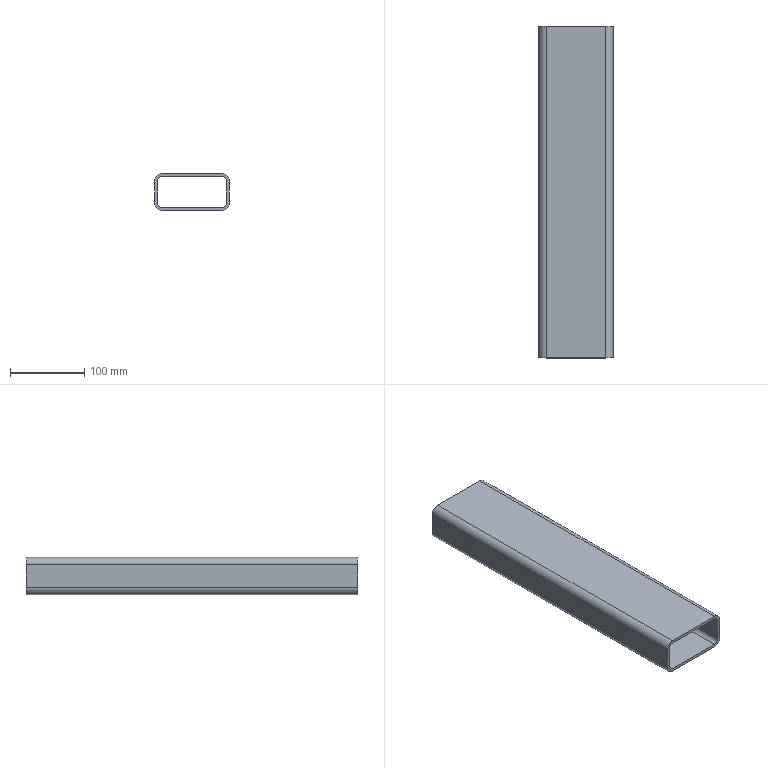Part | SolidWorks | features ExtruThin 1 | 1 solid | 18 faces | box 100 x 446 x 50 mm | volume 482154 mm3 | plane 10 | cylinder 8 | commonest cylinder face diameters 12 x4 20 x4
STEP:
#1=CARTESIAN_POINT('',(50.,223.,-15.));
#2=VERTEX_POINT('',#1);
#3=CARTESIAN_POINT('',(40.,223.,-25.));
#4=VERTEX_POINT('',#3);
#5=CARTESIAN_POINT('',(40.,223.,-15.));
#6=DIRECTION('',(0.,1.,0.));
#7=DIRECTION('',(0.,0.,-1.));
#8=AXIS2_PLACEMENT_3D('',#5,#6,#7);
#9=CIRCLE('',#8,10.);
#10=EDGE_CURVE('',#2,#4,#9,.T.);
#11=ORIENTED_EDGE('',*,*,#10,.T.);
#12=CARTESIAN_POINT('',(-40.,223.,-25.));
#13=VERTEX_POINT('',#12);
#14=CARTESIAN_POINT('',(-40.,223.,-25.));
#15=DIRECTION('',(-1.,0.,0.));
#16=VECTOR('',#15,1000.);
#17=LINE('',#14,#16);
#18=EDGE_CURVE('',#4,#13,#17,.T.);
#19=ORIENTED_EDGE('',*,*,#18,.T.);
#20=CARTESIAN_POINT('',(-50.,223.,-15.));
#21=VERTEX_POINT('',#20);
#22=CARTESIAN_POINT('',(-40.,223.,-15.));
#23=DIRECTION('',(0.,1.,0.));
#24=DIRECTION('',(0.,0.,1.));
#25=AXIS2_PLACEMENT_3D('',#22,#23,#24);
#26=CIRCLE('',#25,10.);
#27=EDGE_CURVE('',#13,#21,#26,.T.);
#28=ORIENTED_EDGE('',*,*,#27,.T.);
#29=CARTESIAN_POINT('',(-50.,223.,15.));
#30=VERTEX_POINT('',#29);
#31=CARTESIAN_POINT('',(-50.,223.,-15.));
#32=DIRECTION('',(0.,0.,1.));
#33=VECTOR('',#32,1000.);
#34=LINE('',#31,#33);
#35=EDGE_CURVE('',#21,#30,#34,.T.);
#36=ORIENTED_EDGE('',*,*,#35,.T.);
#37=CARTESIAN_POINT('',(-40.,223.,25.));
#38=VERTEX_POINT('',#37);
#39=CARTESIAN_POINT('',(-40.,223.,15.));
#40=DIRECTION('',(0.,1.,0.));
#41=DIRECTION('',(0.,0.,1.));
#42=AXIS2_PLACEMENT_3D('',#39,#40,#41);
#43=CIRCLE('',#42,10.);
#44=EDGE_CURVE('',#30,#38,#43,.T.);
#45=ORIENTED_EDGE('',*,*,#44,.T.);
#46=CARTESIAN_POINT('',(40.,223.,25.));
#47=VERTEX_POINT('',#46);
#48=CARTESIAN_POINT('',(-40.,223.,25.));
#49=DIRECTION('',(1.,0.,0.));
#50=VECTOR('',#49,1000.);
#51=LINE('',#48,#50);
#52=EDGE_CURVE('',#38,#47,#51,.T.);
#53=ORIENTED_EDGE('',*,*,#52,.T.);
#54=CARTESIAN_POINT('',(50.,223.,15.));
#55=VERTEX_POINT('',#54);
#56=CARTESIAN_POINT('',(40.,223.,15.));
#57=DIRECTION('',(0.,1.,0.));
#58=DIRECTION('',(0.,0.,1.));
#59=AXIS2_PLACEMENT_3D('',#56,#57,#58);
#60=CIRCLE('',#59,10.);
#61=EDGE_CURVE('',#47,#55,#60,.T.);
#62=ORIENTED_EDGE('',*,*,#61,.T.);
#63=CARTESIAN_POINT('',(50.,223.,-15.));
#64=DIRECTION('',(0.,0.,-1.));
#65=VECTOR('',#64,1000.);
#66=LINE('',#63,#65);
#67=EDGE_CURVE('',#55,#2,#66,.T.);
#68=ORIENTED_EDGE('',*,*,#67,.T.);
#69=EDGE_LOOP('',(#11,#19,#28,#36,#45,#53,#62,#68));
#70=FACE_OUTER_BOUND('',#69,.T.);
#71=CARTESIAN_POINT('',(40.,223.,-21.));
#72=VERTEX_POINT('',#71);
#73=CARTESIAN_POINT('',(-40.,223.,-21.));
#74=VERTEX_POINT('',#73);
#75=CARTESIAN_POINT('',(40.,223.,-21.));
#76=DIRECTION('',(-1.,0.,0.));
#77=VECTOR('',#76,1000.);
#78=LINE('',#75,#77);
#79=EDGE_CURVE('',#72,#74,#78,.T.);
#80=ORIENTED_EDGE('',*,*,#79,.F.);
#81=CARTESIAN_POINT('',(46.,223.,-15.));
#82=VERTEX_POINT('',#81);
#83=CARTESIAN_POINT('',(40.,223.,-15.));
#84=DIRECTION('',(0.,1.,0.));
#85=DIRECTION('',(-1.,0.,0.));
#86=AXIS2_PLACEMENT_3D('',#83,#84,#85);
#87=CIRCLE('',#86,6.);
#88=EDGE_CURVE('',#82,#72,#87,.T.);
#89=ORIENTED_EDGE('',*,*,#88,.F.);
#90=CARTESIAN_POINT('',(46.,223.,15.));
#91=VERTEX_POINT('',#90);
#92=CARTESIAN_POINT('',(46.,223.,-15.));
#93=DIRECTION('',(0.,0.,-1.));
#94=VECTOR('',#93,1000.);
#95=LINE('',#92,#94);
#96=EDGE_CURVE('',#91,#82,#95,.T.);
#97=ORIENTED_EDGE('',*,*,#96,.F.);
#98=CARTESIAN_POINT('',(40.,223.,21.));
#99=VERTEX_POINT('',#98);
#100=CARTESIAN_POINT('',(40.,223.,15.));
#101=DIRECTION('',(0.,1.,0.));
#102=DIRECTION('',(-1.,0.,0.));
#103=AXIS2_PLACEMENT_3D('',#100,#101,#102);
#104=CIRCLE('',#103,6.);
#105=EDGE_CURVE('',#99,#91,#104,.T.);
#106=ORIENTED_EDGE('',*,*,#105,.F.);
#107=CARTESIAN_POINT('',(-40.,223.,21.));
#108=VERTEX_POINT('',#107);
#109=CARTESIAN_POINT('',(40.,223.,21.));
#110=DIRECTION('',(1.,0.,0.));
#111=VECTOR('',#110,1000.);
#112=LINE('',#109,#111);
#113=EDGE_CURVE('',#108,#99,#112,.T.);
#114=ORIENTED_EDGE('',*,*,#113,.F.);
#115=CARTESIAN_POINT('',(-46.,223.,15.));
#116=VERTEX_POINT('',#115);
#117=CARTESIAN_POINT('',(-40.,223.,15.));
#118=DIRECTION('',(0.,1.,0.));
#119=DIRECTION('',(-1.,0.,0.));
#120=AXIS2_PLACEMENT_3D('',#117,#118,#119);
#121=CIRCLE('',#120,6.);
#122=EDGE_CURVE('',#116,#108,#121,.T.);
#123=ORIENTED_EDGE('',*,*,#122,.F.);
#124=CARTESIAN_POINT('',(-46.,223.,-15.));
#125=VERTEX_POINT('',#124);
#126=CARTESIAN_POINT('',(-46.,223.,-15.));
#127=DIRECTION('',(0.,0.,1.));
#128=VECTOR('',#127,1000.);
#129=LINE('',#126,#128);
#130=EDGE_CURVE('',#125,#116,#129,.T.);
#131=ORIENTED_EDGE('',*,*,#130,.F.);
#132=CARTESIAN_POINT('',(-40.,223.,-15.));
#133=DIRECTION('',(0.,1.,0.));
#134=DIRECTION('',(-1.,0.,0.));
#135=AXIS2_PLACEMENT_3D('',#132,#133,#134);
#136=CIRCLE('',#135,6.);
#137=EDGE_CURVE('',#74,#125,#136,.T.);
#138=ORIENTED_EDGE('',*,*,#137,.F.);
#139=EDGE_LOOP('',(#80,#89,#97,#106,#114,#123,#131,#138));
#140=FACE_BOUND('',#139,.T.);
#141=CARTESIAN_POINT('',(40.,223.,-15.));
#142=DIRECTION('',(0.,1.,0.));
#143=DIRECTION('',(0.,0.,1.));
#144=AXIS2_PLACEMENT_3D('',#141,#142,#143);
#145=PLANE('',#144);
#146=ADVANCED_FACE('',(#70,#140),#145,.T.);
#147=CARTESIAN_POINT('',(50.,-223.,-15.));
#148=VERTEX_POINT('',#147);
#149=CARTESIAN_POINT('',(40.,-223.,-25.));
#150=VERTEX_POINT('',#149);
#151=CARTESIAN_POINT('',(40.,-223.,-15.));
#152=DIRECTION('',(0.,1.,0.));
#153=DIRECTION('',(0.,0.,-1.));
#154=AXIS2_PLACEMENT_3D('',#151,#152,#153);
#155=CIRCLE('',#154,10.);
#156=EDGE_CURVE('',#148,#150,#155,.T.);
#157=ORIENTED_EDGE('',*,*,#156,.F.);
#158=CARTESIAN_POINT('',(50.,-223.,15.));
#159=VERTEX_POINT('',#158);
#160=CARTESIAN_POINT('',(50.,-223.,-15.));
#161=DIRECTION('',(0.,0.,-1.));
#162=VECTOR('',#161,1000.);
#163=LINE('',#160,#162);
#164=EDGE_CURVE('',#159,#148,#163,.T.);
#165=ORIENTED_EDGE('',*,*,#164,.F.);
#166=CARTESIAN_POINT('',(40.,-223.,25.));
#167=VERTEX_POINT('',#166);
#168=CARTESIAN_POINT('',(40.,-223.,15.));
#169=DIRECTION('',(0.,1.,0.));
#170=DIRECTION('',(0.,0.,1.));
#171=AXIS2_PLACEMENT_3D('',#168,#169,#170);
#172=CIRCLE('',#171,10.);
#173=EDGE_CURVE('',#167,#159,#172,.T.);
#174=ORIENTED_EDGE('',*,*,#173,.F.);
#175=CARTESIAN_POINT('',(-40.,-223.,25.));
#176=VERTEX_POINT('',#175);
#177=CARTESIAN_POINT('',(-40.,-223.,25.));
#178=DIRECTION('',(1.,0.,0.));
#179=VECTOR('',#178,1000.);
#180=LINE('',#177,#179);
#181=EDGE_CURVE('',#176,#167,#180,.T.);
#182=ORIENTED_EDGE('',*,*,#181,.F.);
#183=CARTESIAN_POINT('',(-50.,-223.,15.));
#184=VERTEX_POINT('',#183);
#185=CARTESIAN_POINT('',(-40.,-223.,15.));
#186=DIRECTION('',(0.,1.,0.));
#187=DIRECTION('',(0.,0.,1.));
#188=AXIS2_PLACEMENT_3D('',#185,#186,#187);
#189=CIRCLE('',#188,10.);
#190=EDGE_CURVE('',#184,#176,#189,.T.);
#191=ORIENTED_EDGE('',*,*,#190,.F.);
#192=CARTESIAN_POINT('',(-50.,-223.,-15.));
#193=VERTEX_POINT('',#192);
#194=CARTESIAN_POINT('',(-50.,-223.,-15.));
#195=DIRECTION('',(0.,0.,1.));
#196=VECTOR('',#195,1000.);
#197=LINE('',#194,#196);
#198=EDGE_CURVE('',#193,#184,#197,.T.);
#199=ORIENTED_EDGE('',*,*,#198,.F.);
#200=CARTESIAN_POINT('',(-40.,-223.,-25.));
#201=VERTEX_POINT('',#200);
#202=CARTESIAN_POINT('',(-40.,-223.,-15.));
#203=DIRECTION('',(0.,1.,0.));
#204=DIRECTION('',(0.,0.,1.));
#205=AXIS2_PLACEMENT_3D('',#202,#203,#204);
#206=CIRCLE('',#205,10.);
#207=EDGE_CURVE('',#201,#193,#206,.T.);
#208=ORIENTED_EDGE('',*,*,#207,.F.);
#209=CARTESIAN_POINT('',(-40.,-223.,-25.));
#210=DIRECTION('',(-1.,0.,0.));
#211=VECTOR('',#210,1000.);
#212=LINE('',#209,#211);
#213=EDGE_CURVE('',#150,#201,#212,.T.);
#214=ORIENTED_EDGE('',*,*,#213,.F.);
#215=EDGE_LOOP('',(#157,#165,#174,#182,#191,#199,#208,#214));
#216=FACE_OUTER_BOUND('',#215,.T.);
#217=CARTESIAN_POINT('',(46.,-223.,-15.));
#218=VERTEX_POINT('',#217);
#219=CARTESIAN_POINT('',(40.,-223.,-21.));
#220=VERTEX_POINT('',#219);
#221=CARTESIAN_POINT('',(40.,-223.,-15.));
#222=DIRECTION('',(0.,1.,0.));
#223=DIRECTION('',(-1.,0.,0.));
#224=AXIS2_PLACEMENT_3D('',#221,#222,#223);
#225=CIRCLE('',#224,6.);
#226=EDGE_CURVE('',#218,#220,#225,.T.);
#227=ORIENTED_EDGE('',*,*,#226,.T.);
#228=CARTESIAN_POINT('',(-40.,-223.,-21.));
#229=VERTEX_POINT('',#228);
#230=CARTESIAN_POINT('',(40.,-223.,-21.));
#231=DIRECTION('',(-1.,0.,0.));
#232=VECTOR('',#231,1000.);
#233=LINE('',#230,#232);
#234=EDGE_CURVE('',#220,#229,#233,.T.);
#235=ORIENTED_EDGE('',*,*,#234,.T.);
#236=CARTESIAN_POINT('',(-46.,-223.,-15.));
#237=VERTEX_POINT('',#236);
#238=CARTESIAN_POINT('',(-40.,-223.,-15.));
#239=DIRECTION('',(0.,1.,0.));
#240=DIRECTION('',(-1.,0.,0.));
#241=AXIS2_PLACEMENT_3D('',#238,#239,#240);
#242=CIRCLE('',#241,6.);
#243=EDGE_CURVE('',#229,#237,#242,.T.);
#244=ORIENTED_EDGE('',*,*,#243,.T.);
#245=CARTESIAN_POINT('',(-46.,-223.,15.));
#246=VERTEX_POINT('',#245);
#247=CARTESIAN_POINT('',(-46.,-223.,-15.));
#248=DIRECTION('',(0.,0.,1.));
#249=VECTOR('',#248,1000.);
#250=LINE('',#247,#249);
#251=EDGE_CURVE('',#237,#246,#250,.T.);
#252=ORIENTED_EDGE('',*,*,#251,.T.);
#253=CARTESIAN_POINT('',(-40.,-223.,21.));
#254=VERTEX_POINT('',#253);
#255=CARTESIAN_POINT('',(-40.,-223.,15.));
#256=DIRECTION('',(0.,1.,0.));
#257=DIRECTION('',(-1.,0.,0.));
#258=AXIS2_PLACEMENT_3D('',#255,#256,#257);
#259=CIRCLE('',#258,6.);
#260=EDGE_CURVE('',#246,#254,#259,.T.);
#261=ORIENTED_EDGE('',*,*,#260,.T.);
#262=CARTESIAN_POINT('',(40.,-223.,21.));
#263=VERTEX_POINT('',#262);
#264=CARTESIAN_POINT('',(40.,-223.,21.));
#265=DIRECTION('',(1.,0.,0.));
#266=VECTOR('',#265,1000.);
#267=LINE('',#264,#266);
#268=EDGE_CURVE('',#254,#263,#267,.T.);
#269=ORIENTED_EDGE('',*,*,#268,.T.);
#270=CARTESIAN_POINT('',(46.,-223.,15.));
#271=VERTEX_POINT('',#270);
#272=CARTESIAN_POINT('',(40.,-223.,15.));
#273=DIRECTION('',(0.,1.,0.));
#274=DIRECTION('',(-1.,0.,0.));
#275=AXIS2_PLACEMENT_3D('',#272,#273,#274);
#276=CIRCLE('',#275,6.);
#277=EDGE_CURVE('',#263,#271,#276,.T.);
#278=ORIENTED_EDGE('',*,*,#277,.T.);
#279=CARTESIAN_POINT('',(46.,-223.,-15.));
#280=DIRECTION('',(0.,0.,-1.));
#281=VECTOR('',#280,1000.);
#282=LINE('',#279,#281);
#283=EDGE_CURVE('',#271,#218,#282,.T.);
#284=ORIENTED_EDGE('',*,*,#283,.T.);
#285=EDGE_LOOP('',(#227,#235,#244,#252,#261,#269,#278,#284));
#286=FACE_BOUND('',#285,.T.);
#287=CARTESIAN_POINT('',(40.,-223.,-15.));
#288=DIRECTION('',(0.,1.,0.));
#289=DIRECTION('',(0.,0.,1.));
#290=AXIS2_PLACEMENT_3D('',#287,#288,#289);
#291=PLANE('',#290);
#292=ADVANCED_FACE('',(#216,#286),#291,.F.);
#293=ORIENTED_EDGE('',*,*,#156,.T.);
#294=CARTESIAN_POINT('',(40.,223.,-25.));
#295=DIRECTION('',(0.,-1.,0.));
#296=VECTOR('',#295,1000.);
#297=LINE('',#294,#296);
#298=EDGE_CURVE('',#4,#150,#297,.T.);
#299=ORIENTED_EDGE('',*,*,#298,.F.);
#300=ORIENTED_EDGE('',*,*,#10,.F.);
#301=CARTESIAN_POINT('',(50.,223.,-15.));
#302=DIRECTION('',(0.,-1.,0.));
#303=VECTOR('',#302,1000.);
#304=LINE('',#301,#303);
#305=EDGE_CURVE('',#2,#148,#304,.T.);
#306=ORIENTED_EDGE('',*,*,#305,.T.);
#307=EDGE_LOOP('',(#293,#299,#300,#306));
#308=FACE_OUTER_BOUND('',#307,.T.);
#309=CARTESIAN_POINT('',(40.,223.,-15.));
#310=DIRECTION('',(0.,-1.,0.));
#311=DIRECTION('',(0.,0.,-1.));
#312=AXIS2_PLACEMENT_3D('',#309,#310,#311);
#313=CYLINDRICAL_SURFACE('',#312,10.);
#314=ADVANCED_FACE('',(#308),#313,.T.);
#315=ORIENTED_EDGE('',*,*,#213,.T.);
#316=CARTESIAN_POINT('',(-40.,223.,-25.));
#317=DIRECTION('',(0.,-1.,0.));
#318=VECTOR('',#317,1000.);
#319=LINE('',#316,#318);
#320=EDGE_CURVE('',#13,#201,#319,.T.);
#321=ORIENTED_EDGE('',*,*,#320,.F.);
#322=ORIENTED_EDGE('',*,*,#18,.F.);
#323=ORIENTED_EDGE('',*,*,#298,.T.);
#324=EDGE_LOOP('',(#315,#321,#322,#323));
#325=FACE_OUTER_BOUND('',#324,.T.);
#326=CARTESIAN_POINT('',(-40.,223.,-25.));
#327=DIRECTION('',(0.,0.,1.));
#328=DIRECTION('',(1.,0.,0.));
#329=AXIS2_PLACEMENT_3D('',#326,#327,#328);
#330=PLANE('',#329);
#331=ADVANCED_FACE('',(#325),#330,.F.);
#332=ORIENTED_EDGE('',*,*,#207,.T.);
#333=CARTESIAN_POINT('',(-50.,223.,-15.));
#334=DIRECTION('',(0.,-1.,0.));
#335=VECTOR('',#334,1000.);
#336=LINE('',#333,#335);
#337=EDGE_CURVE('',#21,#193,#336,.T.);
#338=ORIENTED_EDGE('',*,*,#337,.F.);
#339=ORIENTED_EDGE('',*,*,#27,.F.);
#340=ORIENTED_EDGE('',*,*,#320,.T.);
#341=EDGE_LOOP('',(#332,#338,#339,#340));
#342=FACE_OUTER_BOUND('',#341,.T.);
#343=CARTESIAN_POINT('',(-40.,223.,-15.));
#344=DIRECTION('',(0.,-1.,0.));
#345=DIRECTION('',(0.,0.,-1.));
#346=AXIS2_PLACEMENT_3D('',#343,#344,#345);
#347=CYLINDRICAL_SURFACE('',#346,10.);
#348=ADVANCED_FACE('',(#342),#347,.T.);
#349=ORIENTED_EDGE('',*,*,#198,.T.);
#350=CARTESIAN_POINT('',(-50.,223.,15.));
#351=DIRECTION('',(0.,-1.,0.));
#352=VECTOR('',#351,1000.);
#353=LINE('',#350,#352);
#354=EDGE_CURVE('',#30,#184,#353,.T.);
#355=ORIENTED_EDGE('',*,*,#354,.F.);
#356=ORIENTED_EDGE('',*,*,#35,.F.);
#357=ORIENTED_EDGE('',*,*,#337,.T.);
#358=EDGE_LOOP('',(#349,#355,#356,#357));
#359=FACE_OUTER_BOUND('',#358,.T.);
#360=CARTESIAN_POINT('',(-50.,223.,-15.));
#361=DIRECTION('',(1.,0.,0.));
#362=DIRECTION('',(0.,0.,-1.));
#363=AXIS2_PLACEMENT_3D('',#360,#361,#362);
#364=PLANE('',#363);
#365=ADVANCED_FACE('',(#359),#364,.F.);
#366=ORIENTED_EDGE('',*,*,#190,.T.);
#367=CARTESIAN_POINT('',(-40.,223.,25.));
#368=DIRECTION('',(0.,-1.,0.));
#369=VECTOR('',#368,1000.);
#370=LINE('',#367,#369);
#371=EDGE_CURVE('',#38,#176,#370,.T.);
#372=ORIENTED_EDGE('',*,*,#371,.F.);
#373=ORIENTED_EDGE('',*,*,#44,.F.);
#374=ORIENTED_EDGE('',*,*,#354,.T.);
#375=EDGE_LOOP('',(#366,#372,#373,#374));
#376=FACE_OUTER_BOUND('',#375,.T.);
#377=CARTESIAN_POINT('',(-40.,223.,15.));
#378=DIRECTION('',(0.,-1.,0.));
#379=DIRECTION('',(0.,0.,-1.));
#380=AXIS2_PLACEMENT_3D('',#377,#378,#379);
#381=CYLINDRICAL_SURFACE('',#380,10.);
#382=ADVANCED_FACE('',(#376),#381,.T.);
#383=ORIENTED_EDGE('',*,*,#181,.T.);
#384=CARTESIAN_POINT('',(40.,223.,25.));
#385=DIRECTION('',(0.,-1.,0.));
#386=VECTOR('',#385,1000.);
#387=LINE('',#384,#386);
#388=EDGE_CURVE('',#47,#167,#387,.T.);
#389=ORIENTED_EDGE('',*,*,#388,.F.);
#390=ORIENTED_EDGE('',*,*,#52,.F.);
#391=ORIENTED_EDGE('',*,*,#371,.T.);
#392=EDGE_LOOP('',(#383,#389,#390,#391));
#393=FACE_OUTER_BOUND('',#392,.T.);
#394=CARTESIAN_POINT('',(-40.,223.,25.));
#395=DIRECTION('',(0.,0.,-1.));
#396=DIRECTION('',(-1.,0.,0.));
#397=AXIS2_PLACEMENT_3D('',#394,#395,#396);
#398=PLANE('',#397);
#399=ADVANCED_FACE('',(#393),#398,.F.);
#400=ORIENTED_EDGE('',*,*,#173,.T.);
#401=CARTESIAN_POINT('',(50.,223.,15.));
#402=DIRECTION('',(0.,-1.,0.));
#403=VECTOR('',#402,1000.);
#404=LINE('',#401,#403);
#405=EDGE_CURVE('',#55,#159,#404,.T.);
#406=ORIENTED_EDGE('',*,*,#405,.F.);
#407=ORIENTED_EDGE('',*,*,#61,.F.);
#408=ORIENTED_EDGE('',*,*,#388,.T.);
#409=EDGE_LOOP('',(#400,#406,#407,#408));
#410=FACE_OUTER_BOUND('',#409,.T.);
#411=CARTESIAN_POINT('',(40.,223.,15.));
#412=DIRECTION('',(0.,-1.,0.));
#413=DIRECTION('',(0.,0.,-1.));
#414=AXIS2_PLACEMENT_3D('',#411,#412,#413);
#415=CYLINDRICAL_SURFACE('',#414,10.);
#416=ADVANCED_FACE('',(#410),#415,.T.);
#417=ORIENTED_EDGE('',*,*,#164,.T.);
#418=ORIENTED_EDGE('',*,*,#305,.F.);
#419=ORIENTED_EDGE('',*,*,#67,.F.);
#420=ORIENTED_EDGE('',*,*,#405,.T.);
#421=EDGE_LOOP('',(#417,#418,#419,#420));
#422=FACE_OUTER_BOUND('',#421,.T.);
#423=CARTESIAN_POINT('',(50.,223.,-15.));
#424=DIRECTION('',(-1.,0.,0.));
#425=DIRECTION('',(0.,0.,1.));
#426=AXIS2_PLACEMENT_3D('',#423,#424,#425);
#427=PLANE('',#426);
#428=ADVANCED_FACE('',(#422),#427,.F.);
#429=ORIENTED_EDGE('',*,*,#226,.F.);
#430=CARTESIAN_POINT('',(46.,223.,-15.));
#431=DIRECTION('',(0.,-1.,0.));
#432=VECTOR('',#431,1000.);
#433=LINE('',#430,#432);
#434=EDGE_CURVE('',#82,#218,#433,.T.);
#435=ORIENTED_EDGE('',*,*,#434,.F.);
#436=ORIENTED_EDGE('',*,*,#88,.T.);
#437=CARTESIAN_POINT('',(40.,223.,-21.));
#438=DIRECTION('',(0.,-1.,0.));
#439=VECTOR('',#438,1000.);
#440=LINE('',#437,#439);
#441=EDGE_CURVE('',#72,#220,#440,.T.);
#442=ORIENTED_EDGE('',*,*,#441,.T.);
#443=EDGE_LOOP('',(#429,#435,#436,#442));
#444=FACE_OUTER_BOUND('',#443,.T.);
#445=CARTESIAN_POINT('',(40.,223.,-15.));
#446=DIRECTION('',(0.,-1.,0.));
#447=DIRECTION('',(0.,0.,-1.));
#448=AXIS2_PLACEMENT_3D('',#445,#446,#447);
#449=CYLINDRICAL_SURFACE('',#448,6.);
#450=ADVANCED_FACE('',(#444),#449,.F.);
#451=ORIENTED_EDGE('',*,*,#234,.F.);
#452=ORIENTED_EDGE('',*,*,#441,.F.);
#453=ORIENTED_EDGE('',*,*,#79,.T.);
#454=CARTESIAN_POINT('',(-40.,223.,-21.));
#455=DIRECTION('',(0.,-1.,0.));
#456=VECTOR('',#455,1000.);
#457=LINE('',#454,#456);
#458=EDGE_CURVE('',#74,#229,#457,.T.);
#459=ORIENTED_EDGE('',*,*,#458,.T.);
#460=EDGE_LOOP('',(#451,#452,#453,#459));
#461=FACE_OUTER_BOUND('',#460,.T.);
#462=CARTESIAN_POINT('',(40.,223.,-21.));
#463=DIRECTION('',(0.,0.,1.));
#464=DIRECTION('',(1.,0.,0.));
#465=AXIS2_PLACEMENT_3D('',#462,#463,#464);
#466=PLANE('',#465);
#467=ADVANCED_FACE('',(#461),#466,.T.);
#468=ORIENTED_EDGE('',*,*,#243,.F.);
#469=ORIENTED_EDGE('',*,*,#458,.F.);
#470=ORIENTED_EDGE('',*,*,#137,.T.);
#471=CARTESIAN_POINT('',(-46.,223.,-15.));
#472=DIRECTION('',(0.,-1.,0.));
#473=VECTOR('',#472,1000.);
#474=LINE('',#471,#473);
#475=EDGE_CURVE('',#125,#237,#474,.T.);
#476=ORIENTED_EDGE('',*,*,#475,.T.);
#477=EDGE_LOOP('',(#468,#469,#470,#476));
#478=FACE_OUTER_BOUND('',#477,.T.);
#479=CARTESIAN_POINT('',(-40.,223.,-15.));
#480=DIRECTION('',(0.,-1.,0.));
#481=DIRECTION('',(0.,0.,-1.));
#482=AXIS2_PLACEMENT_3D('',#479,#480,#481);
#483=CYLINDRICAL_SURFACE('',#482,6.);
#484=ADVANCED_FACE('',(#478),#483,.F.);
#485=ORIENTED_EDGE('',*,*,#251,.F.);
#486=ORIENTED_EDGE('',*,*,#475,.F.);
#487=ORIENTED_EDGE('',*,*,#130,.T.);
#488=CARTESIAN_POINT('',(-46.,223.,15.));
#489=DIRECTION('',(0.,-1.,0.));
#490=VECTOR('',#489,1000.);
#491=LINE('',#488,#490);
#492=EDGE_CURVE('',#116,#246,#491,.T.);
#493=ORIENTED_EDGE('',*,*,#492,.T.);
#494=EDGE_LOOP('',(#485,#486,#487,#493));
#495=FACE_OUTER_BOUND('',#494,.T.);
#496=CARTESIAN_POINT('',(-46.,223.,-15.));
#497=DIRECTION('',(1.,0.,0.));
#498=DIRECTION('',(0.,0.,-1.));
#499=AXIS2_PLACEMENT_3D('',#496,#497,#498);
#500=PLANE('',#499);
#501=ADVANCED_FACE('',(#495),#500,.T.);
#502=ORIENTED_EDGE('',*,*,#260,.F.);
#503=ORIENTED_EDGE('',*,*,#492,.F.);
#504=ORIENTED_EDGE('',*,*,#122,.T.);
#505=CARTESIAN_POINT('',(-40.,223.,21.));
#506=DIRECTION('',(0.,-1.,0.));
#507=VECTOR('',#506,1000.);
#508=LINE('',#505,#507);
#509=EDGE_CURVE('',#108,#254,#508,.T.);
#510=ORIENTED_EDGE('',*,*,#509,.T.);
#511=EDGE_LOOP('',(#502,#503,#504,#510));
#512=FACE_OUTER_BOUND('',#511,.T.);
#513=CARTESIAN_POINT('',(-40.,223.,15.));
#514=DIRECTION('',(0.,-1.,0.));
#515=DIRECTION('',(0.,0.,-1.));
#516=AXIS2_PLACEMENT_3D('',#513,#514,#515);
#517=CYLINDRICAL_SURFACE('',#516,6.);
#518=ADVANCED_FACE('',(#512),#517,.F.);
#519=ORIENTED_EDGE('',*,*,#268,.F.);
#520=ORIENTED_EDGE('',*,*,#509,.F.);
#521=ORIENTED_EDGE('',*,*,#113,.T.);
#522=CARTESIAN_POINT('',(40.,223.,21.));
#523=DIRECTION('',(0.,-1.,0.));
#524=VECTOR('',#523,1000.);
#525=LINE('',#522,#524);
#526=EDGE_CURVE('',#99,#263,#525,.T.);
#527=ORIENTED_EDGE('',*,*,#526,.T.);
#528=EDGE_LOOP('',(#519,#520,#521,#527));
#529=FACE_OUTER_BOUND('',#528,.T.);
#530=CARTESIAN_POINT('',(40.,223.,21.));
#531=DIRECTION('',(0.,0.,-1.));
#532=DIRECTION('',(-1.,0.,0.));
#533=AXIS2_PLACEMENT_3D('',#530,#531,#532);
#534=PLANE('',#533);
#535=ADVANCED_FACE('',(#529),#534,.T.);
#536=ORIENTED_EDGE('',*,*,#277,.F.);
#537=ORIENTED_EDGE('',*,*,#526,.F.);
#538=ORIENTED_EDGE('',*,*,#105,.T.);
#539=CARTESIAN_POINT('',(46.,223.,15.));
#540=DIRECTION('',(0.,-1.,0.));
#541=VECTOR('',#540,1000.);
#542=LINE('',#539,#541);
#543=EDGE_CURVE('',#91,#271,#542,.T.);
#544=ORIENTED_EDGE('',*,*,#543,.T.);
#545=EDGE_LOOP('',(#536,#537,#538,#544));
#546=FACE_OUTER_BOUND('',#545,.T.);
#547=CARTESIAN_POINT('',(40.,223.,15.));
#548=DIRECTION('',(0.,-1.,0.));
#549=DIRECTION('',(0.,0.,-1.));
#550=AXIS2_PLACEMENT_3D('',#547,#548,#549);
#551=CYLINDRICAL_SURFACE('',#550,6.);
#552=ADVANCED_FACE('',(#546),#551,.F.);
#553=ORIENTED_EDGE('',*,*,#283,.F.);
#554=ORIENTED_EDGE('',*,*,#543,.F.);
#555=ORIENTED_EDGE('',*,*,#96,.T.);
#556=ORIENTED_EDGE('',*,*,#434,.T.);
#557=EDGE_LOOP('',(#553,#554,#555,#556));
#558=FACE_OUTER_BOUND('',#557,.T.);
#559=CARTESIAN_POINT('',(46.,223.,-15.));
#560=DIRECTION('',(-1.,0.,0.));
#561=DIRECTION('',(0.,0.,1.));
#562=AXIS2_PLACEMENT_3D('',#559,#560,#561);
#563=PLANE('',#562);
#564=ADVANCED_FACE('',(#558),#563,.T.);
#565=CLOSED_SHELL('',(#146,#292,#314,#331,#348,#365,#382,#399,#416,#428,#450,#467,#484,#501,#518,#535,#552,#564));
#566=MANIFOLD_SOLID_BREP('',#565);
#567=CARTESIAN_POINT('',(0.,0.,0.));
#568=DIRECTION('',(0.,0.,1.));
#569=DIRECTION('',(1.,0.,0.));
#570=AXIS2_PLACEMENT_3D('',#567,#568,#569);
#571=(LENGTH_UNIT()NAMED_UNIT(*)SI_UNIT(.MILLI.,.METRE.));
#572=UNCERTAINTY_MEASURE_WITH_UNIT(LENGTH_MEASURE(0.00001),#571,'','');
#573=(NAMED_UNIT(*)PLANE_ANGLE_UNIT()SI_UNIT($,.RADIAN.));
#574=(NAMED_UNIT(*)SI_UNIT($,.STERADIAN.)SOLID_ANGLE_UNIT());
#575=(GEOMETRIC_REPRESENTATION_CONTEXT(3)GLOBAL_UNCERTAINTY_ASSIGNED_CONTEXT((#572))GLOBAL_UNIT_ASSIGNED_CONTEXT((#571,#573,#574))REPRESENTATION_CONTEXT('',''));
#576=ADVANCED_BREP_SHAPE_REPRESENTATION('',(#566,#570),#575);